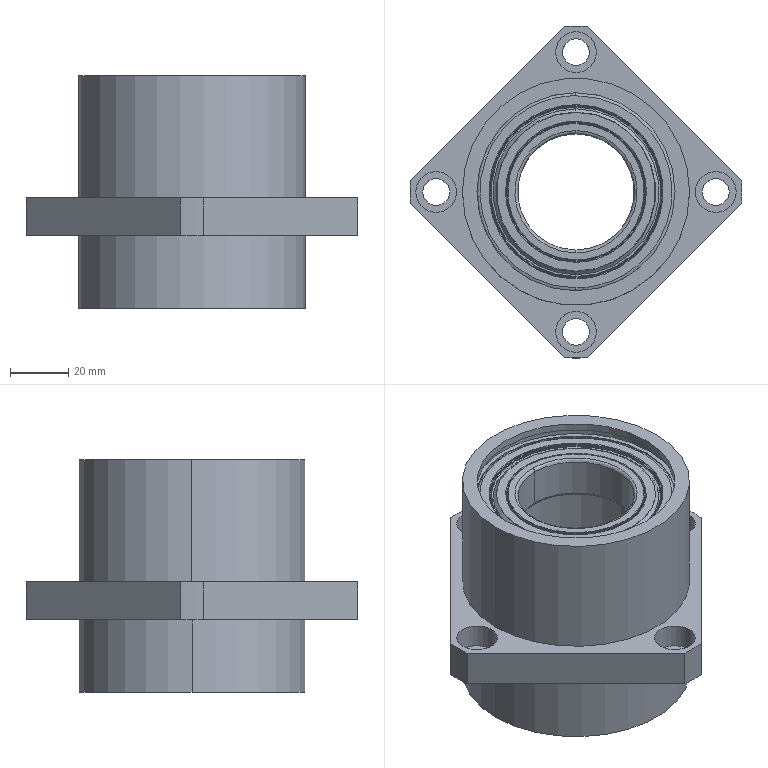Part | SolidWorks | features BaseBody 3 | 3 solids | 331 faces | box 114 x 114 x 80 mm | volume 207286 mm3 | spline 106 | cylinder 103 | cone 80 | plane 42 | commonest cylinder face diameters 68 x12 9.2 x8 14 x8 46.3 x8 47.2 x8 47.8 x8